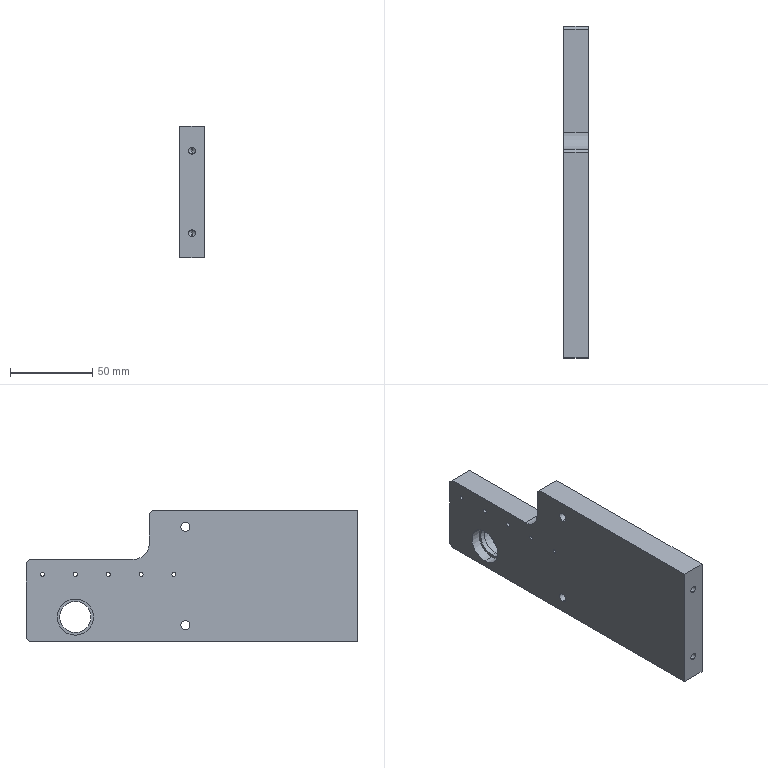Part | SolidWorks | features HoleWzd 4, ICE 3, Chamfer 1, Cut 1, Extrusion 1 | 1 solid | 63 faces | box 15 x 202 x 80 mm | volume 199416 mm3 | cylinder 36 | plane 19 | cone 8 | commonest cylinder face diameters 2.5 x10 4.2 x4 5 x4 5.5 x4 10 x4 22 x4